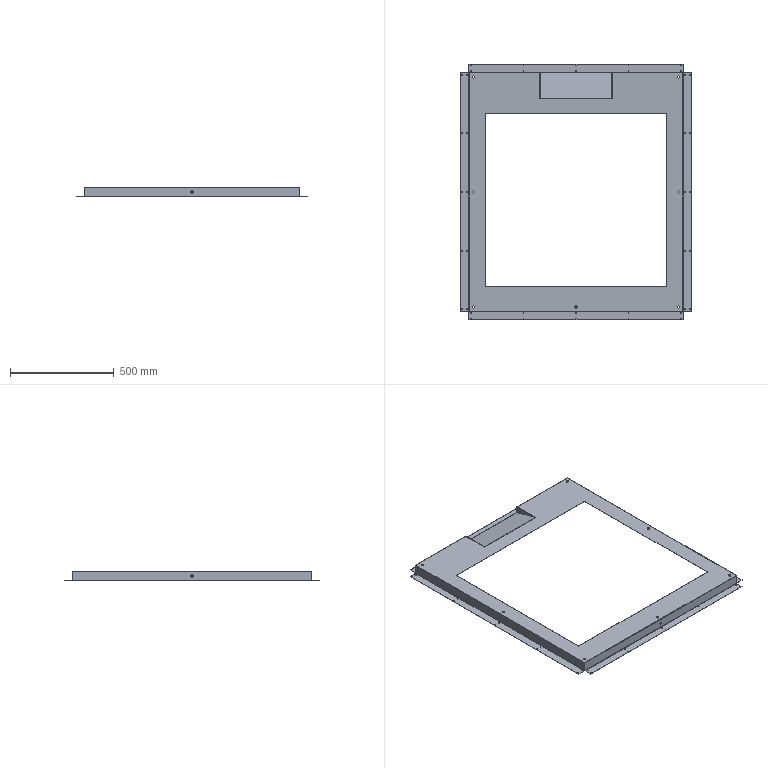Part | SolidWorks | 2 solids | 204 faces | box 1113 x 1233 x 48 mm | volume 830275 mm3 | cylinder 122 | plane 70 | spline 12 | commonest cylinder face diameters 4.2 x80 11 x14 0.4 x11 2.4 x11 10 x6